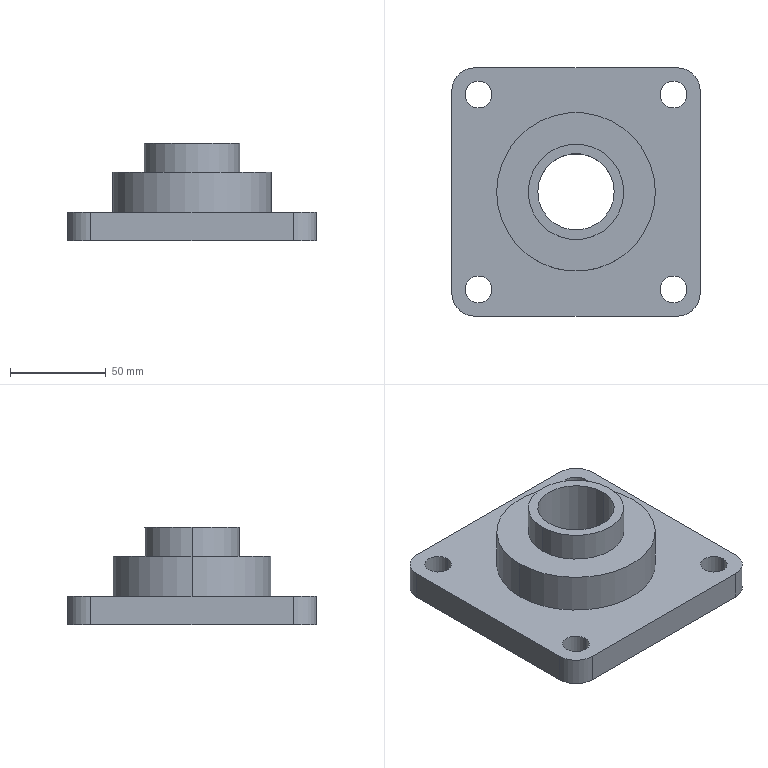Part | STEP file | UCF208 bearing housing XG | 1 solid | 32 faces | box 130 x 130 x 51.2 mm | volume 310699 mm3 | cylinder 22 | plane 10 | commonest cylinder face diameters 14 x8 24 x4 50 x4 40 x2 70 x2 83 x2